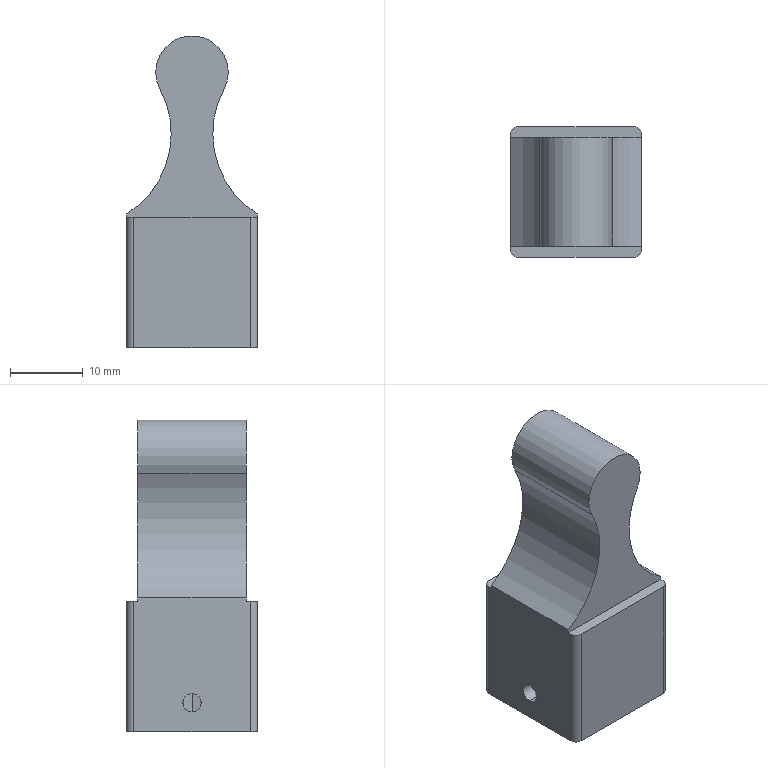Part | STEP file | Seal sleeve 1 | 1 solid | 21 faces | box 18 x 18 x 43 mm | volume 8232 mm3 | cylinder 11 | plane 10 | commonest cylinder face diameters 2 x4 10 x3 2.5 x2 26 x2